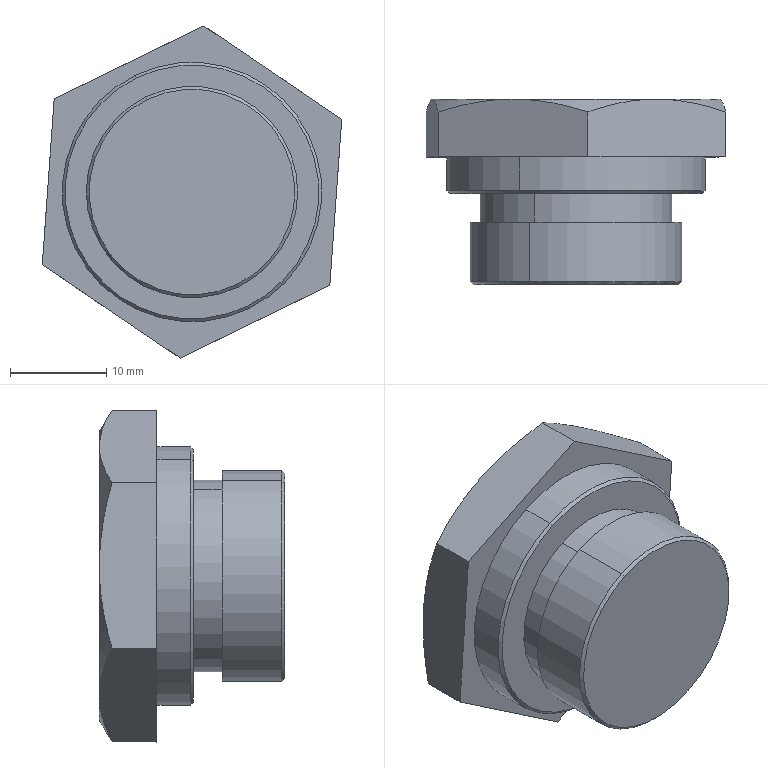Part | SolidWorks | features BaseBody 1 | 1 solid | 27 faces | box 31.164 x 19.3 x 34.552 mm | volume 10229 mm3 | plane 11 | cone 10 | cylinder 6 | commonest cylinder face diameters 20 x2 22 x2 27 x2
STEP:
#1=CARTESIAN_POINT('',(-39.66,84.896,-168.446));
#2=VERTEX_POINT('',#1);
#3=CARTESIAN_POINT('',(-49.266,84.896,-148.654));
#4=VERTEX_POINT('',#3);
#5=CARTESIAN_POINT('',(-44.463,84.896,-158.55));
#6=DIRECTION('',(0.,1.,0.));
#7=DIRECTION('',(0.4367,0.,-0.8996));
#8=AXIS2_PLACEMENT_3D('',#5,#6,#7);
#9=CIRCLE('',#8,11.);
#10=EDGE_CURVE('',#2,#4,#9,.T.);
#11=ORIENTED_EDGE('',*,*,#10,.T.);
#12=CARTESIAN_POINT('',(-49.266,91.096,-148.654));
#13=VERTEX_POINT('',#12);
#14=CARTESIAN_POINT('',(-49.266,153.67,-148.654));
#15=DIRECTION('',(0.,1.,0.));
#16=VECTOR('',#15,1000.);
#17=LINE('',#14,#16);
#18=EDGE_CURVE('',#4,#13,#17,.T.);
#19=ORIENTED_EDGE('',*,*,#18,.T.);
#20=CARTESIAN_POINT('',(-39.66,91.096,-168.446));
#21=VERTEX_POINT('',#20);
#22=CARTESIAN_POINT('',(-44.463,91.096,-158.55));
#23=DIRECTION('',(0.,1.,0.));
#24=DIRECTION('',(0.4367,0.,-0.8996));
#25=AXIS2_PLACEMENT_3D('',#22,#23,#24);
#26=CIRCLE('',#25,11.);
#27=EDGE_CURVE('',#21,#13,#26,.T.);
#28=ORIENTED_EDGE('',*,*,#27,.F.);
#29=CARTESIAN_POINT('',(-39.66,153.67,-168.446));
#30=DIRECTION('',(0.,1.,0.));
#31=VECTOR('',#30,1000.);
#32=LINE('',#29,#31);
#33=EDGE_CURVE('',#2,#21,#32,.T.);
#34=ORIENTED_EDGE('',*,*,#33,.F.);
#35=EDGE_LOOP('',(#11,#19,#28,#34));
#36=FACE_OUTER_BOUND('',#35,.T.);
#37=CARTESIAN_POINT('',(-44.463,153.67,-158.55));
#38=DIRECTION('',(0.,1.,0.));
#39=DIRECTION('',(0.4367,0.,-0.8996));
#40=AXIS2_PLACEMENT_3D('',#37,#38,#39);
#41=CYLINDRICAL_SURFACE('',#40,11.);
#42=ADVANCED_FACE('',(#36),#41,.T.);
#43=CARTESIAN_POINT('',(-40.096,91.096,-167.546));
#44=VERTEX_POINT('',#43);
#45=CARTESIAN_POINT('',(-48.829,91.096,-149.554));
#46=VERTEX_POINT('',#45);
#47=CARTESIAN_POINT('',(-44.463,91.096,-158.55));
#48=DIRECTION('',(0.,1.,0.));
#49=DIRECTION('',(0.4367,0.,-0.8996));
#50=AXIS2_PLACEMENT_3D('',#47,#48,#49);
#51=CIRCLE('',#50,10.);
#52=EDGE_CURVE('',#44,#46,#51,.T.);
#53=ORIENTED_EDGE('',*,*,#52,.T.);
#54=CARTESIAN_POINT('',(-48.829,94.096,-149.554));
#55=VERTEX_POINT('',#54);
#56=CARTESIAN_POINT('',(-48.829,153.67,-149.554));
#57=DIRECTION('',(0.,1.,0.));
#58=VECTOR('',#57,1000.);
#59=LINE('',#56,#58);
#60=EDGE_CURVE('',#46,#55,#59,.T.);
#61=ORIENTED_EDGE('',*,*,#60,.T.);
#62=CARTESIAN_POINT('',(-40.096,94.096,-167.546));
#63=VERTEX_POINT('',#62);
#64=CARTESIAN_POINT('',(-44.463,94.096,-158.55));
#65=DIRECTION('',(0.,1.,0.));
#66=DIRECTION('',(0.4367,0.,-0.8996));
#67=AXIS2_PLACEMENT_3D('',#64,#65,#66);
#68=CIRCLE('',#67,10.);
#69=EDGE_CURVE('',#63,#55,#68,.T.);
#70=ORIENTED_EDGE('',*,*,#69,.F.);
#71=CARTESIAN_POINT('',(-40.096,153.67,-167.546));
#72=DIRECTION('',(0.,1.,0.));
#73=VECTOR('',#72,1000.);
#74=LINE('',#71,#73);
#75=EDGE_CURVE('',#44,#63,#74,.T.);
#76=ORIENTED_EDGE('',*,*,#75,.F.);
#77=EDGE_LOOP('',(#53,#61,#70,#76));
#78=FACE_OUTER_BOUND('',#77,.T.);
#79=CARTESIAN_POINT('',(-44.463,153.67,-158.55));
#80=DIRECTION('',(0.,1.,0.));
#81=DIRECTION('',(0.4367,0.,-0.8996));
#82=AXIS2_PLACEMENT_3D('',#79,#80,#81);
#83=CYLINDRICAL_SURFACE('',#82,10.);
#84=ADVANCED_FACE('',(#78),#83,.T.);
#85=CARTESIAN_POINT('',(-38.699,94.096,-170.425));
#86=VERTEX_POINT('',#85);
#87=CARTESIAN_POINT('',(-50.227,94.096,-146.675));
#88=VERTEX_POINT('',#87);
#89=CARTESIAN_POINT('',(-44.463,94.096,-158.55));
#90=DIRECTION('',(0.,1.,0.));
#91=DIRECTION('',(0.4367,0.,-0.8996));
#92=AXIS2_PLACEMENT_3D('',#89,#90,#91);
#93=CIRCLE('',#92,13.2);
#94=EDGE_CURVE('',#86,#88,#93,.T.);
#95=ORIENTED_EDGE('',*,*,#94,.T.);
#96=CARTESIAN_POINT('',(-50.358,94.396,-146.405));
#97=VERTEX_POINT('',#96);
#98=CARTESIAN_POINT('',(-50.227,94.096,-146.675));
#99=DIRECTION('',(-0.3088,0.7071,0.6361));
#100=VECTOR('',#99,1000.);
#101=LINE('',#98,#100);
#102=EDGE_CURVE('',#88,#97,#101,.T.);
#103=ORIENTED_EDGE('',*,*,#102,.T.);
#104=CARTESIAN_POINT('',(-38.568,94.396,-170.695));
#105=VERTEX_POINT('',#104);
#106=CARTESIAN_POINT('',(-44.463,94.396,-158.55));
#107=DIRECTION('',(0.,1.,0.));
#108=DIRECTION('',(0.4367,0.,-0.8996));
#109=AXIS2_PLACEMENT_3D('',#106,#107,#108);
#110=CIRCLE('',#109,13.5);
#111=EDGE_CURVE('',#105,#97,#110,.T.);
#112=ORIENTED_EDGE('',*,*,#111,.F.);
#113=CARTESIAN_POINT('',(-38.699,94.096,-170.425));
#114=DIRECTION('',(0.3088,0.7071,-0.6361));
#115=VECTOR('',#114,1000.);
#116=LINE('',#113,#115);
#117=EDGE_CURVE('',#86,#105,#116,.T.);
#118=ORIENTED_EDGE('',*,*,#117,.F.);
#119=EDGE_LOOP('',(#95,#103,#112,#118));
#120=FACE_OUTER_BOUND('',#119,.T.);
#121=CARTESIAN_POINT('',(-44.463,94.096,-158.55));
#122=DIRECTION('',(0.,1.,0.));
#123=DIRECTION('',(0.4367,0.,-0.8996));
#124=AXIS2_PLACEMENT_3D('',#121,#122,#123);
#125=CONICAL_SURFACE('',#124,13.2,0.7854);
#126=ADVANCED_FACE('',(#120),#125,.T.);
#127=ORIENTED_EDGE('',*,*,#111,.T.);
#128=CARTESIAN_POINT('',(-50.358,97.896,-146.405));
#129=VERTEX_POINT('',#128);
#130=CARTESIAN_POINT('',(-50.358,153.67,-146.405));
#131=DIRECTION('',(0.,1.,0.));
#132=VECTOR('',#131,1000.);
#133=LINE('',#130,#132);
#134=EDGE_CURVE('',#97,#129,#133,.T.);
#135=ORIENTED_EDGE('',*,*,#134,.T.);
#136=CARTESIAN_POINT('',(-38.568,97.896,-170.695));
#137=VERTEX_POINT('',#136);
#138=CARTESIAN_POINT('',(-44.463,97.896,-158.55));
#139=DIRECTION('',(0.,1.,0.));
#140=DIRECTION('',(0.4367,0.,-0.8996));
#141=AXIS2_PLACEMENT_3D('',#138,#139,#140);
#142=CIRCLE('',#141,13.5);
#143=EDGE_CURVE('',#137,#129,#142,.T.);
#144=ORIENTED_EDGE('',*,*,#143,.F.);
#145=CARTESIAN_POINT('',(-38.568,153.67,-170.695));
#146=DIRECTION('',(0.,1.,0.));
#147=VECTOR('',#146,1000.);
#148=LINE('',#145,#147);
#149=EDGE_CURVE('',#105,#137,#148,.T.);
#150=ORIENTED_EDGE('',*,*,#149,.F.);
#151=EDGE_LOOP('',(#127,#135,#144,#150));
#152=FACE_OUTER_BOUND('',#151,.T.);
#153=CARTESIAN_POINT('',(-44.463,153.67,-158.55));
#154=DIRECTION('',(0.,1.,0.));
#155=DIRECTION('',(0.4367,0.,-0.8996));
#156=AXIS2_PLACEMENT_3D('',#153,#154,#155);
#157=CYLINDRICAL_SURFACE('',#156,13.5);
#158=ADVANCED_FACE('',(#152),#157,.T.);
#159=CARTESIAN_POINT('',(-49.135,84.596,-148.924));
#160=VERTEX_POINT('',#159);
#161=CARTESIAN_POINT('',(-39.791,84.596,-168.176));
#162=VERTEX_POINT('',#161);
#163=CARTESIAN_POINT('',(-44.463,84.596,-158.55));
#164=DIRECTION('',(0.,-1.,0.));
#165=DIRECTION('',(0.4367,0.,-0.8996));
#166=AXIS2_PLACEMENT_3D('',#163,#164,#165);
#167=CIRCLE('',#166,10.7);
#168=EDGE_CURVE('',#160,#162,#167,.T.);
#169=ORIENTED_EDGE('',*,*,#168,.F.);
#170=CARTESIAN_POINT('',(-49.266,84.896,-148.654));
#171=DIRECTION('',(-0.3088,0.7071,0.6361));
#172=VECTOR('',#171,1000.);
#173=LINE('',#170,#172);
#174=EDGE_CURVE('',#160,#4,#173,.T.);
#175=ORIENTED_EDGE('',*,*,#174,.T.);
#176=ORIENTED_EDGE('',*,*,#10,.F.);
#177=CARTESIAN_POINT('',(-39.66,84.896,-168.446));
#178=DIRECTION('',(0.3088,0.7071,-0.6361));
#179=VECTOR('',#178,1000.);
#180=LINE('',#177,#179);
#181=EDGE_CURVE('',#162,#2,#180,.T.);
#182=ORIENTED_EDGE('',*,*,#181,.F.);
#183=EDGE_LOOP('',(#169,#175,#176,#182));
#184=FACE_OUTER_BOUND('',#183,.T.);
#185=CARTESIAN_POINT('',(-44.463,84.896,-158.55));
#186=DIRECTION('',(0.,1.,0.));
#187=DIRECTION('',(0.4367,0.,-0.8996));
#188=AXIS2_PLACEMENT_3D('',#185,#186,#187);
#189=CONICAL_SURFACE('',#188,11.,0.7854);
#190=ADVANCED_FACE('',(#184),#189,.T.);
#191=ORIENTED_EDGE('',*,*,#174,.F.);
#192=CARTESIAN_POINT('',(-44.463,84.596,-158.55));
#193=DIRECTION('',(0.,-1.,0.));
#194=DIRECTION('',(0.4367,0.,-0.8996));
#195=AXIS2_PLACEMENT_3D('',#192,#193,#194);
#196=CIRCLE('',#195,10.7);
#197=EDGE_CURVE('',#162,#160,#196,.T.);
#198=ORIENTED_EDGE('',*,*,#197,.F.);
#199=ORIENTED_EDGE('',*,*,#181,.T.);
#200=CARTESIAN_POINT('',(-44.463,84.896,-158.55));
#201=DIRECTION('',(0.,1.,0.));
#202=DIRECTION('',(0.4367,0.,-0.8996));
#203=AXIS2_PLACEMENT_3D('',#200,#201,#202);
#204=CIRCLE('',#203,11.);
#205=EDGE_CURVE('',#4,#2,#204,.T.);
#206=ORIENTED_EDGE('',*,*,#205,.F.);
#207=EDGE_LOOP('',(#191,#198,#199,#206));
#208=FACE_OUTER_BOUND('',#207,.T.);
#209=CARTESIAN_POINT('',(-44.463,84.896,-158.55));
#210=DIRECTION('',(0.,1.,0.));
#211=DIRECTION('',(0.4367,0.,-0.8996));
#212=AXIS2_PLACEMENT_3D('',#209,#210,#211);
#213=CONICAL_SURFACE('',#212,11.,0.7854);
#214=ADVANCED_FACE('',(#208),#213,.T.);
#215=CARTESIAN_POINT('',(-51.013,103.896,-145.056));
#216=VERTEX_POINT('',#215);
#217=CARTESIAN_POINT('',(-59.424,103.896,-157.475));
#218=VERTEX_POINT('',#217);
#219=CARTESIAN_POINT('',(-44.463,103.896,-158.55));
#220=DIRECTION('',(0.,-1.,0.));
#221=DIRECTION('',(-0.4367,0.,0.8996));
#222=AXIS2_PLACEMENT_3D('',#219,#220,#221);
#223=CIRCLE('',#222,15.);
#224=EDGE_CURVE('',#216,#218,#223,.T.);
#225=ORIENTED_EDGE('',*,*,#224,.F.);
#226=CARTESIAN_POINT('',(-36.051,103.896,-146.13));
#227=VERTEX_POINT('',#226);
#228=CARTESIAN_POINT('',(-44.463,103.896,-158.55));
#229=DIRECTION('',(0.,-1.,0.));
#230=DIRECTION('',(-0.4367,0.,0.8996));
#231=AXIS2_PLACEMENT_3D('',#228,#229,#230);
#232=CIRCLE('',#231,15.);
#233=EDGE_CURVE('',#227,#216,#232,.T.);
#234=ORIENTED_EDGE('',*,*,#233,.F.);
#235=CARTESIAN_POINT('',(-29.501,103.896,-159.625));
#236=VERTEX_POINT('',#235);
#237=CARTESIAN_POINT('',(-44.463,103.896,-158.55));
#238=DIRECTION('',(0.,-1.,0.));
#239=DIRECTION('',(-0.4367,0.,0.8996));
#240=AXIS2_PLACEMENT_3D('',#237,#238,#239);
#241=CIRCLE('',#240,15.);
#242=EDGE_CURVE('',#236,#227,#241,.T.);
#243=ORIENTED_EDGE('',*,*,#242,.F.);
#244=CARTESIAN_POINT('',(-37.913,103.896,-172.044));
#245=VERTEX_POINT('',#244);
#246=CARTESIAN_POINT('',(-44.463,103.896,-158.55));
#247=DIRECTION('',(0.,-1.,0.));
#248=DIRECTION('',(-0.4367,0.,0.8996));
#249=AXIS2_PLACEMENT_3D('',#246,#247,#248);
#250=CIRCLE('',#249,15.);
#251=EDGE_CURVE('',#245,#236,#250,.T.);
#252=ORIENTED_EDGE('',*,*,#251,.F.);
#253=CARTESIAN_POINT('',(-52.874,103.896,-170.97));
#254=VERTEX_POINT('',#253);
#255=CARTESIAN_POINT('',(-44.463,103.896,-158.55));
#256=DIRECTION('',(0.,1.,0.));
#257=DIRECTION('',(0.4367,0.,-0.8996));
#258=AXIS2_PLACEMENT_3D('',#255,#256,#257);
#259=CIRCLE('',#258,15.);
#260=EDGE_CURVE('',#245,#254,#259,.T.);
#261=ORIENTED_EDGE('',*,*,#260,.T.);
#262=CARTESIAN_POINT('',(-44.463,103.896,-158.55));
#263=DIRECTION('',(0.,-1.,0.));
#264=DIRECTION('',(-0.4367,0.,0.8996));
#265=AXIS2_PLACEMENT_3D('',#262,#263,#264);
#266=CIRCLE('',#265,15.);
#267=EDGE_CURVE('',#218,#254,#266,.T.);
#268=ORIENTED_EDGE('',*,*,#267,.F.);
#269=EDGE_LOOP('',(#225,#234,#243,#252,#261,#268));
#270=FACE_OUTER_BOUND('',#269,.T.);
#271=CARTESIAN_POINT('',(-44.463,103.896,-158.55));
#272=DIRECTION('',(0.,-1.,0.));
#273=DIRECTION('',(-1.,0.,0.));
#274=AXIS2_PLACEMENT_3D('',#271,#272,#273);
#275=PLANE('',#274);
#276=ADVANCED_FACE('',(#270),#275,.F.);
#277=ORIENTED_EDGE('',*,*,#224,.T.);
#278=CARTESIAN_POINT('',(-58.804,102.556,-148.837));
#279=VERTEX_POINT('',#278);
#280=CARTESIAN_POINT('',(-58.804,102.556,-148.837));
#281=CARTESIAN_POINT('',(-58.905,102.965,-150.248));
#282=CARTESIAN_POINT('',(-59.007,103.302,-151.67));
#283=CARTESIAN_POINT('',(-59.214,103.768,-154.547));
#284=CARTESIAN_POINT('',(-59.318,103.896,-156.001));
#285=CARTESIAN_POINT('',(-59.424,103.896,-157.475));
#286=B_SPLINE_CURVE_WITH_KNOTS('',3,(#280,#281,#282,#283,#284,#285),.UNSPECIFIED.,.F.,.F.,(4,2,4),(0.,0.004382,0.008763),.UNSPECIFIED.);
#287=EDGE_CURVE('',#279,#218,#286,.T.);
#288=ORIENTED_EDGE('',*,*,#287,.F.);
#289=CARTESIAN_POINT('',(-51.013,103.896,-145.056));
#290=CARTESIAN_POINT('',(-52.342,103.896,-145.701));
#291=CARTESIAN_POINT('',(-53.654,103.768,-146.338));
#292=CARTESIAN_POINT('',(-56.248,103.302,-147.597));
#293=CARTESIAN_POINT('',(-57.531,102.965,-148.219));
#294=CARTESIAN_POINT('',(-58.804,102.556,-148.837));
#295=B_SPLINE_CURVE_WITH_KNOTS('',3,(#289,#290,#291,#292,#293,#294),.UNSPECIFIED.,.F.,.F.,(4,2,4),(0.,0.004382,0.008763),.UNSPECIFIED.);
#296=EDGE_CURVE('',#216,#279,#295,.T.);
#297=ORIENTED_EDGE('',*,*,#296,.F.);
#298=EDGE_LOOP('',(#277,#288,#297));
#299=FACE_OUTER_BOUND('',#298,.T.);
#300=CARTESIAN_POINT('',(-44.463,103.896,-158.55));
#301=DIRECTION('',(0.,-1.,0.));
#302=DIRECTION('',(-0.4367,0.,0.8996));
#303=AXIS2_PLACEMENT_3D('',#300,#301,#302);
#304=CONICAL_SURFACE('',#303,15.,1.047);
#305=ADVANCED_FACE('',(#299),#304,.T.);
#306=CARTESIAN_POINT('',(-60.045,102.556,-166.113));
#307=VERTEX_POINT('',#306);
#308=CARTESIAN_POINT('',(-59.424,103.896,-157.475));
#309=CARTESIAN_POINT('',(-59.53,103.896,-158.949));
#310=CARTESIAN_POINT('',(-59.635,103.768,-160.404));
#311=CARTESIAN_POINT('',(-59.841,103.302,-163.28));
#312=CARTESIAN_POINT('',(-59.944,102.965,-164.702));
#313=CARTESIAN_POINT('',(-60.045,102.556,-166.113));
#314=B_SPLINE_CURVE_WITH_KNOTS('',3,(#308,#309,#310,#311,#312,#313),.UNSPECIFIED.,.F.,.F.,(4,2,4),(0.,0.004382,0.008763),.UNSPECIFIED.);
#315=EDGE_CURVE('',#218,#307,#314,.T.);
#316=ORIENTED_EDGE('',*,*,#315,.F.);
#317=ORIENTED_EDGE('',*,*,#267,.T.);
#318=CARTESIAN_POINT('',(-60.045,102.556,-166.113));
#319=CARTESIAN_POINT('',(-58.874,102.965,-166.906));
#320=CARTESIAN_POINT('',(-57.693,103.302,-167.706));
#321=CARTESIAN_POINT('',(-55.305,103.768,-169.323));
#322=CARTESIAN_POINT('',(-54.098,103.896,-170.141));
#323=CARTESIAN_POINT('',(-52.874,103.896,-170.97));
#324=B_SPLINE_CURVE_WITH_KNOTS('',3,(#318,#319,#320,#321,#322,#323),.UNSPECIFIED.,.F.,.F.,(4,2,4),(0.,0.004382,0.008763),.UNSPECIFIED.);
#325=EDGE_CURVE('',#307,#254,#324,.T.);
#326=ORIENTED_EDGE('',*,*,#325,.F.);
#327=EDGE_LOOP('',(#316,#317,#326));
#328=FACE_OUTER_BOUND('',#327,.T.);
#329=CARTESIAN_POINT('',(-44.463,103.896,-158.55));
#330=DIRECTION('',(0.,-1.,0.));
#331=DIRECTION('',(-0.4367,0.,0.8996));
#332=AXIS2_PLACEMENT_3D('',#329,#330,#331);
#333=CONICAL_SURFACE('',#332,15.,1.047);
#334=ADVANCED_FACE('',(#328),#333,.T.);
#335=ORIENTED_EDGE('',*,*,#260,.F.);
#336=CARTESIAN_POINT('',(-45.704,102.556,-175.826));
#337=VERTEX_POINT('',#336);
#338=CARTESIAN_POINT('',(-45.704,102.556,-175.826));
#339=CARTESIAN_POINT('',(-44.431,102.965,-175.208));
#340=CARTESIAN_POINT('',(-43.149,103.302,-174.586));
#341=CARTESIAN_POINT('',(-40.554,103.768,-173.326));
#342=CARTESIAN_POINT('',(-39.243,103.896,-172.69));
#343=CARTESIAN_POINT('',(-37.913,103.896,-172.044));
#344=B_SPLINE_CURVE_WITH_KNOTS('',3,(#338,#339,#340,#341,#342,#343),.UNSPECIFIED.,.F.,.F.,(4,2,4),(0.,0.004382,0.008763),.UNSPECIFIED.);
#345=EDGE_CURVE('',#337,#245,#344,.T.);
#346=ORIENTED_EDGE('',*,*,#345,.F.);
#347=CARTESIAN_POINT('',(-52.874,103.896,-170.97));
#348=CARTESIAN_POINT('',(-51.651,103.896,-171.798));
#349=CARTESIAN_POINT('',(-50.444,103.768,-172.616));
#350=CARTESIAN_POINT('',(-48.056,103.302,-174.233));
#351=CARTESIAN_POINT('',(-46.875,102.965,-175.033));
#352=CARTESIAN_POINT('',(-45.704,102.556,-175.826));
#353=B_SPLINE_CURVE_WITH_KNOTS('',3,(#347,#348,#349,#350,#351,#352),.UNSPECIFIED.,.F.,.F.,(4,2,4),(0.,0.004382,0.008763),.UNSPECIFIED.);
#354=EDGE_CURVE('',#254,#337,#353,.T.);
#355=ORIENTED_EDGE('',*,*,#354,.F.);
#356=EDGE_LOOP('',(#335,#346,#355));
#357=FACE_OUTER_BOUND('',#356,.T.);
#358=CARTESIAN_POINT('',(-44.463,103.896,-158.55));
#359=DIRECTION('',(0.,-1.,0.));
#360=DIRECTION('',(-0.4367,0.,0.8996));
#361=AXIS2_PLACEMENT_3D('',#358,#359,#360);
#362=CONICAL_SURFACE('',#361,15.,1.047);
#363=ADVANCED_FACE('',(#357),#362,.T.);
#364=ORIENTED_EDGE('',*,*,#251,.T.);
#365=CARTESIAN_POINT('',(-30.122,102.556,-168.263));
#366=VERTEX_POINT('',#365);
#367=CARTESIAN_POINT('',(-30.122,102.556,-168.263));
#368=CARTESIAN_POINT('',(-30.021,102.965,-166.852));
#369=CARTESIAN_POINT('',(-29.918,103.302,-165.43));
#370=CARTESIAN_POINT('',(-29.712,103.768,-162.553));
#371=CARTESIAN_POINT('',(-29.607,103.896,-161.099));
#372=CARTESIAN_POINT('',(-29.501,103.896,-159.625));
#373=B_SPLINE_CURVE_WITH_KNOTS('',3,(#367,#368,#369,#370,#371,#372),.UNSPECIFIED.,.F.,.F.,(4,2,4),(0.,0.004382,0.008763),.UNSPECIFIED.);
#374=EDGE_CURVE('',#366,#236,#373,.T.);
#375=ORIENTED_EDGE('',*,*,#374,.F.);
#376=CARTESIAN_POINT('',(-37.913,103.896,-172.044));
#377=CARTESIAN_POINT('',(-36.583,103.896,-171.399));
#378=CARTESIAN_POINT('',(-35.272,103.768,-170.762));
#379=CARTESIAN_POINT('',(-32.677,103.302,-169.503));
#380=CARTESIAN_POINT('',(-31.395,102.965,-168.881));
#381=CARTESIAN_POINT('',(-30.122,102.556,-168.263));
#382=B_SPLINE_CURVE_WITH_KNOTS('',3,(#376,#377,#378,#379,#380,#381),.UNSPECIFIED.,.F.,.F.,(4,2,4),(0.,0.004382,0.008763),.UNSPECIFIED.);
#383=EDGE_CURVE('',#245,#366,#382,.T.);
#384=ORIENTED_EDGE('',*,*,#383,.F.);
#385=EDGE_LOOP('',(#364,#375,#384));
#386=FACE_OUTER_BOUND('',#385,.T.);
#387=CARTESIAN_POINT('',(-44.463,103.896,-158.55));
#388=DIRECTION('',(0.,-1.,0.));
#389=DIRECTION('',(-0.4367,0.,0.8996));
#390=AXIS2_PLACEMENT_3D('',#387,#388,#389);
#391=CONICAL_SURFACE('',#390,15.,1.047);
#392=ADVANCED_FACE('',(#386),#391,.T.);
#393=ORIENTED_EDGE('',*,*,#242,.T.);
#394=CARTESIAN_POINT('',(-28.881,102.556,-150.987));
#395=VERTEX_POINT('',#394);
#396=CARTESIAN_POINT('',(-28.881,102.556,-150.987));
#397=CARTESIAN_POINT('',(-30.052,102.965,-150.194));
#398=CARTESIAN_POINT('',(-31.233,103.302,-149.394));
#399=CARTESIAN_POINT('',(-33.62,103.768,-147.777));
#400=CARTESIAN_POINT('',(-34.828,103.896,-146.959));
#401=CARTESIAN_POINT('',(-36.051,103.896,-146.13));
#402=B_SPLINE_CURVE_WITH_KNOTS('',3,(#396,#397,#398,#399,#400,#401),.UNSPECIFIED.,.F.,.F.,(4,2,4),(0.,0.004382,0.008763),.UNSPECIFIED.);
#403=EDGE_CURVE('',#395,#227,#402,.T.);
#404=ORIENTED_EDGE('',*,*,#403,.F.);
#405=CARTESIAN_POINT('',(-29.501,103.896,-159.625));
#406=CARTESIAN_POINT('',(-29.396,103.896,-158.151));
#407=CARTESIAN_POINT('',(-29.291,103.768,-156.696));
#408=CARTESIAN_POINT('',(-29.084,103.302,-153.82));
#409=CARTESIAN_POINT('',(-28.982,102.965,-152.398));
#410=CARTESIAN_POINT('',(-28.881,102.556,-150.987));
#411=B_SPLINE_CURVE_WITH_KNOTS('',3,(#405,#406,#407,#408,#409,#410),.UNSPECIFIED.,.F.,.F.,(4,2,4),(0.,0.004382,0.008763),.UNSPECIFIED.);
#412=EDGE_CURVE('',#236,#395,#411,.T.);
#413=ORIENTED_EDGE('',*,*,#412,.F.);
#414=EDGE_LOOP('',(#393,#404,#413));
#415=FACE_OUTER_BOUND('',#414,.T.);
#416=CARTESIAN_POINT('',(-44.463,103.896,-158.55));
#417=DIRECTION('',(0.,-1.,0.));
#418=DIRECTION('',(-0.4367,0.,0.8996));
#419=AXIS2_PLACEMENT_3D('',#416,#417,#418);
#420=CONICAL_SURFACE('',#419,15.,1.047);
#421=ADVANCED_FACE('',(#415),#420,.T.);
#422=ORIENTED_EDGE('',*,*,#233,.T.);
#423=CARTESIAN_POINT('',(-43.222,102.556,-141.274));
#424=VERTEX_POINT('',#423);
#425=CARTESIAN_POINT('',(-43.222,102.556,-141.274));
#426=CARTESIAN_POINT('',(-44.494,102.965,-141.892));
#427=CARTESIAN_POINT('',(-45.777,103.302,-142.514));
#428=CARTESIAN_POINT('',(-48.371,103.768,-143.774));
#429=CARTESIAN_POINT('',(-49.683,103.896,-144.41));
#430=CARTESIAN_POINT('',(-51.013,103.896,-145.056));
#431=B_SPLINE_CURVE_WITH_KNOTS('',3,(#425,#426,#427,#428,#429,#430),.UNSPECIFIED.,.F.,.F.,(4,2,4),(0.,0.004382,0.008763),.UNSPECIFIED.);
#432=EDGE_CURVE('',#424,#216,#431,.T.);
#433=ORIENTED_EDGE('',*,*,#432,.F.);
#434=CARTESIAN_POINT('',(-36.051,103.896,-146.13));
#435=CARTESIAN_POINT('',(-37.275,103.896,-145.302));
#436=CARTESIAN_POINT('',(-38.482,103.768,-144.484));
#437=CARTESIAN_POINT('',(-40.87,103.302,-142.867));
#438=CARTESIAN_POINT('',(-42.05,102.965,-142.067));
#439=CARTESIAN_POINT('',(-43.222,102.556,-141.274));
#440=B_SPLINE_CURVE_WITH_KNOTS('',3,(#434,#435,#436,#437,#438,#439),.UNSPECIFIED.,.F.,.F.,(4,2,4),(0.,0.004382,0.008763),.UNSPECIFIED.);
#441=EDGE_CURVE('',#227,#424,#440,.T.);
#442=ORIENTED_EDGE('',*,*,#441,.F.);
#443=EDGE_LOOP('',(#422,#433,#442));
#444=FACE_OUTER_BOUND('',#443,.T.);
#445=CARTESIAN_POINT('',(-44.463,103.896,-158.55));
#446=DIRECTION('',(0.,-1.,0.));
#447=DIRECTION('',(-0.4367,0.,0.8996));
#448=AXIS2_PLACEMENT_3D('',#445,#446,#447);
#449=CONICAL_SURFACE('',#448,15.,1.047);
#450=ADVANCED_FACE('',(#444),#449,.T.);
#451=ORIENTED_EDGE('',*,*,#143,.T.);
#452=CARTESIAN_POINT('',(-44.463,97.896,-158.55));
#453=DIRECTION('',(0.,1.,0.));
#454=DIRECTION('',(0.4367,0.,-0.8996));
#455=AXIS2_PLACEMENT_3D('',#452,#453,#454);
#456=CIRCLE('',#455,13.5);
#457=EDGE_CURVE('',#129,#137,#456,.T.);
#458=ORIENTED_EDGE('',*,*,#457,.T.);
#459=EDGE_LOOP('',(#451,#458));
#460=FACE_BOUND('',#459,.T.);
#461=CARTESIAN_POINT('',(-58.804,97.896,-148.837));
#462=VERTEX_POINT('',#461);
#463=CARTESIAN_POINT('',(-60.045,97.896,-166.113));
#464=VERTEX_POINT('',#463);
#465=CARTESIAN_POINT('',(-60.045,97.896,-166.113));
#466=DIRECTION('',(-0.07166,0.,-0.9974));
#467=VECTOR('',#466,1000.);
#468=LINE('',#465,#467);
#469=EDGE_CURVE('',#462,#464,#468,.T.);
#470=ORIENTED_EDGE('',*,*,#469,.T.);
#471=CARTESIAN_POINT('',(-45.704,97.896,-175.826));
#472=VERTEX_POINT('',#471);
#473=CARTESIAN_POINT('',(-45.704,97.896,-175.826));
#474=DIRECTION('',(0.828,0.,-0.5608));
#475=VECTOR('',#474,1000.);
#476=LINE('',#473,#475);
#477=EDGE_CURVE('',#464,#472,#476,.T.);
#478=ORIENTED_EDGE('',*,*,#477,.T.);
#479=CARTESIAN_POINT('',(-30.122,97.896,-168.263));
#480=VERTEX_POINT('',#479);
#481=CARTESIAN_POINT('',(-30.122,97.896,-168.263));
#482=DIRECTION('',(0.8996,0.,0.4367));
#483=VECTOR('',#482,1000.);
#484=LINE('',#481,#483);
#485=EDGE_CURVE('',#472,#480,#484,.T.);
#486=ORIENTED_EDGE('',*,*,#485,.T.);
#487=CARTESIAN_POINT('',(-28.881,97.896,-150.987));
#488=VERTEX_POINT('',#487);
#489=CARTESIAN_POINT('',(-28.881,97.896,-150.987));
#490=DIRECTION('',(0.07166,0.,0.9974));
#491=VECTOR('',#490,1000.);
#492=LINE('',#489,#491);
#493=EDGE_CURVE('',#480,#488,#492,.T.);
#494=ORIENTED_EDGE('',*,*,#493,.T.);
#495=CARTESIAN_POINT('',(-43.222,97.896,-141.274));
#496=VERTEX_POINT('',#495);
#497=CARTESIAN_POINT('',(-43.222,97.896,-141.274));
#498=DIRECTION('',(-0.828,0.,0.5608));
#499=VECTOR('',#498,1000.);
#500=LINE('',#497,#499);
#501=EDGE_CURVE('',#488,#496,#500,.T.);
#502=ORIENTED_EDGE('',*,*,#501,.T.);
#503=CARTESIAN_POINT('',(-58.804,97.896,-148.837));
#504=DIRECTION('',(-0.8996,0.,-0.4367));
#505=VECTOR('',#504,1000.);
#506=LINE('',#503,#505);
#507=EDGE_CURVE('',#496,#462,#506,.T.);
#508=ORIENTED_EDGE('',*,*,#507,.T.);
#509=EDGE_LOOP('',(#470,#478,#486,#494,#502,#508));
#510=FACE_OUTER_BOUND('',#509,.T.);
#511=CARTESIAN_POINT('',(-57.957,97.896,-165.1));
#512=DIRECTION('',(0.,1.,0.));
#513=DIRECTION('',(1.,0.,0.));
#514=AXIS2_PLACEMENT_3D('',#511,#512,#513);
#515=PLANE('',#514);
#516=ADVANCED_FACE('',(#460,#510),#515,.F.);
#517=ORIENTED_EDGE('',*,*,#134,.F.);
#518=CARTESIAN_POINT('',(-44.463,94.396,-158.55));
#519=DIRECTION('',(0.,1.,0.));
#520=DIRECTION('',(0.4367,0.,-0.8996));
#521=AXIS2_PLACEMENT_3D('',#518,#519,#520);
#522=CIRCLE('',#521,13.5);
#523=EDGE_CURVE('',#97,#105,#522,.T.);
#524=ORIENTED_EDGE('',*,*,#523,.T.);
#525=ORIENTED_EDGE('',*,*,#149,.T.);
#526=ORIENTED_EDGE('',*,*,#457,.F.);
#527=EDGE_LOOP('',(#517,#524,#525,#526));
#528=FACE_OUTER_BOUND('',#527,.T.);
#529=CARTESIAN_POINT('',(-44.463,153.67,-158.55));
#530=DIRECTION('',(0.,1.,0.));
#531=DIRECTION('',(0.4367,0.,-0.8996));
#532=AXIS2_PLACEMENT_3D('',#529,#530,#531);
#533=CYLINDRICAL_SURFACE('',#532,13.5);
#534=ADVANCED_FACE('',(#528),#533,.T.);
#535=ORIENTED_EDGE('',*,*,#102,.F.);
#536=CARTESIAN_POINT('',(-44.463,94.096,-158.55));
#537=DIRECTION('',(0.,1.,0.));
#538=DIRECTION('',(0.4367,0.,-0.8996));
#539=AXIS2_PLACEMENT_3D('',#536,#537,#538);
#540=CIRCLE('',#539,13.2);
#541=EDGE_CURVE('',#88,#86,#540,.T.);
#542=ORIENTED_EDGE('',*,*,#541,.T.);
#543=ORIENTED_EDGE('',*,*,#117,.T.);
#544=ORIENTED_EDGE('',*,*,#523,.F.);
#545=EDGE_LOOP('',(#535,#542,#543,#544));
#546=FACE_OUTER_BOUND('',#545,.T.);
#547=CARTESIAN_POINT('',(-44.463,94.096,-158.55));
#548=DIRECTION('',(0.,1.,0.));
#549=DIRECTION('',(0.4367,0.,-0.8996));
#550=AXIS2_PLACEMENT_3D('',#547,#548,#549);
#551=CONICAL_SURFACE('',#550,13.2,0.7854);
#552=ADVANCED_FACE('',(#546),#551,.T.);
#553=ORIENTED_EDGE('',*,*,#69,.T.);
#554=CARTESIAN_POINT('',(-44.463,94.096,-158.55));
#555=DIRECTION('',(0.,1.,0.));
#556=DIRECTION('',(0.4367,0.,-0.8996));
#557=AXIS2_PLACEMENT_3D('',#554,#555,#556);
#558=CIRCLE('',#557,10.);
#559=EDGE_CURVE('',#55,#63,#558,.T.);
#560=ORIENTED_EDGE('',*,*,#559,.T.);
#561=EDGE_LOOP('',(#553,#560));
#562=FACE_BOUND('',#561,.T.);
#563=ORIENTED_EDGE('',*,*,#94,.F.);
#564=ORIENTED_EDGE('',*,*,#541,.F.);
#565=EDGE_LOOP('',(#563,#564));
#566=FACE_OUTER_BOUND('',#565,.T.);
#567=CARTESIAN_POINT('',(-56.338,94.096,-164.314));
#568=DIRECTION('',(0.,1.,0.));
#569=DIRECTION('',(1.,0.,0.));
#570=AXIS2_PLACEMENT_3D('',#567,#568,#569);
#571=PLANE('',#570);
#572=ADVANCED_FACE('',(#562,#566),#571,.F.);
#573=ORIENTED_EDGE('',*,*,#60,.F.);
#574=CARTESIAN_POINT('',(-44.463,91.096,-158.55));
#575=DIRECTION('',(0.,1.,0.));
#576=DIRECTION('',(0.4367,0.,-0.8996));
#577=AXIS2_PLACEMENT_3D('',#574,#575,#576);
#578=CIRCLE('',#577,10.);
#579=EDGE_CURVE('',#46,#44,#578,.T.);
#580=ORIENTED_EDGE('',*,*,#579,.T.);
#581=ORIENTED_EDGE('',*,*,#75,.T.);
#582=ORIENTED_EDGE('',*,*,#559,.F.);
#583=EDGE_LOOP('',(#573,#580,#581,#582));
#584=FACE_OUTER_BOUND('',#583,.T.);
#585=CARTESIAN_POINT('',(-44.463,153.67,-158.55));
#586=DIRECTION('',(0.,1.,0.));
#587=DIRECTION('',(0.4367,0.,-0.8996));
#588=AXIS2_PLACEMENT_3D('',#585,#586,#587);
#589=CYLINDRICAL_SURFACE('',#588,10.);
#590=ADVANCED_FACE('',(#584),#589,.T.);
#591=ORIENTED_EDGE('',*,*,#27,.T.);
#592=CARTESIAN_POINT('',(-44.463,91.096,-158.55));
#593=DIRECTION('',(0.,1.,0.));
#594=DIRECTION('',(0.4367,0.,-0.8996));
#595=AXIS2_PLACEMENT_3D('',#592,#593,#594);
#596=CIRCLE('',#595,11.);
#597=EDGE_CURVE('',#13,#21,#596,.T.);
#598=ORIENTED_EDGE('',*,*,#597,.T.);
#599=EDGE_LOOP('',(#591,#598));
#600=FACE_OUTER_BOUND('',#599,.T.);
#601=ORIENTED_EDGE('',*,*,#52,.F.);
#602=ORIENTED_EDGE('',*,*,#579,.F.);
#603=EDGE_LOOP('',(#601,#602));
#604=FACE_BOUND('',#603,.T.);
#605=CARTESIAN_POINT('',(-53.459,91.096,-162.917));
#606=DIRECTION('',(0.,-1.,0.));
#607=DIRECTION('',(-1.,0.,0.));
#608=AXIS2_PLACEMENT_3D('',#605,#606,#607);
#609=PLANE('',#608);
#610=ADVANCED_FACE('',(#600,#604),#609,.F.);
#611=ORIENTED_EDGE('',*,*,#18,.F.);
#612=ORIENTED_EDGE('',*,*,#205,.T.);
#613=ORIENTED_EDGE('',*,*,#33,.T.);
#614=ORIENTED_EDGE('',*,*,#597,.F.);
#615=EDGE_LOOP('',(#611,#612,#613,#614));
#616=FACE_OUTER_BOUND('',#615,.T.);
#617=CARTESIAN_POINT('',(-44.463,153.67,-158.55));
#618=DIRECTION('',(0.,1.,0.));
#619=DIRECTION('',(0.4367,0.,-0.8996));
#620=AXIS2_PLACEMENT_3D('',#617,#618,#619);
#621=CYLINDRICAL_SURFACE('',#620,11.);
#622=ADVANCED_FACE('',(#616),#621,.T.);
#623=ORIENTED_EDGE('',*,*,#197,.T.);
#624=ORIENTED_EDGE('',*,*,#168,.T.);
#625=EDGE_LOOP('',(#623,#624));
#626=FACE_OUTER_BOUND('',#625,.T.);
#627=CARTESIAN_POINT('',(-54.359,84.596,-163.353));
#628=DIRECTION('',(0.,1.,0.));
#629=DIRECTION('',(1.,0.,0.));
#630=AXIS2_PLACEMENT_3D('',#627,#628,#629);
#631=PLANE('',#630);
#632=ADVANCED_FACE('',(#626),#631,.F.);
#633=CARTESIAN_POINT('',(-58.804,52.07,-148.837));
#634=DIRECTION('',(0.,1.,0.));
#635=VECTOR('',#634,1000.);
#636=LINE('',#633,#635);
#637=EDGE_CURVE('',#462,#279,#636,.T.);
#638=ORIENTED_EDGE('',*,*,#637,.T.);
#639=ORIENTED_EDGE('',*,*,#287,.T.);
#640=ORIENTED_EDGE('',*,*,#315,.T.);
#641=CARTESIAN_POINT('',(-60.045,52.07,-166.113));
#642=DIRECTION('',(0.,1.,0.));
#643=VECTOR('',#642,1000.);
#644=LINE('',#641,#643);
#645=EDGE_CURVE('',#464,#307,#644,.T.);
#646=ORIENTED_EDGE('',*,*,#645,.F.);
#647=ORIENTED_EDGE('',*,*,#469,.F.);
#648=EDGE_LOOP('',(#638,#639,#640,#646,#647));
#649=FACE_OUTER_BOUND('',#648,.T.);
#650=CARTESIAN_POINT('',(-60.045,52.07,-166.113));
#651=DIRECTION('',(-0.9974,0.,0.07166));
#652=DIRECTION('',(0.,1.,0.));
#653=AXIS2_PLACEMENT_3D('',#650,#651,#652);
#654=PLANE('',#653);
#655=ADVANCED_FACE('',(#649),#654,.T.);
#656=CARTESIAN_POINT('',(-43.222,52.07,-141.274));
#657=DIRECTION('',(0.,1.,0.));
#658=VECTOR('',#657,1000.);
#659=LINE('',#656,#658);
#660=EDGE_CURVE('',#496,#424,#659,.T.);
#661=ORIENTED_EDGE('',*,*,#660,.T.);
#662=ORIENTED_EDGE('',*,*,#432,.T.);
#663=ORIENTED_EDGE('',*,*,#296,.T.);
#664=ORIENTED_EDGE('',*,*,#637,.F.);
#665=ORIENTED_EDGE('',*,*,#507,.F.);
#666=EDGE_LOOP('',(#661,#662,#663,#664,#665));
#667=FACE_OUTER_BOUND('',#666,.T.);
#668=CARTESIAN_POINT('',(-58.804,52.07,-148.837));
#669=DIRECTION('',(-0.4367,0.,0.8996));
#670=DIRECTION('',(0.,1.,0.));
#671=AXIS2_PLACEMENT_3D('',#668,#669,#670);
#672=PLANE('',#671);
#673=ADVANCED_FACE('',(#667),#672,.T.);
#674=CARTESIAN_POINT('',(-28.881,52.07,-150.987));
#675=DIRECTION('',(0.,1.,0.));
#676=VECTOR('',#675,1000.);
#677=LINE('',#674,#676);
#678=EDGE_CURVE('',#488,#395,#677,.T.);
#679=ORIENTED_EDGE('',*,*,#678,.T.);
#680=ORIENTED_EDGE('',*,*,#403,.T.);
#681=ORIENTED_EDGE('',*,*,#441,.T.);
#682=ORIENTED_EDGE('',*,*,#660,.F.);
#683=ORIENTED_EDGE('',*,*,#501,.F.);
#684=EDGE_LOOP('',(#679,#680,#681,#682,#683));
#685=FACE_OUTER_BOUND('',#684,.T.);
#686=CARTESIAN_POINT('',(-43.222,52.07,-141.274));
#687=DIRECTION('',(0.5608,0.,0.828));
#688=DIRECTION('',(0.,-1.,0.));
#689=AXIS2_PLACEMENT_3D('',#686,#687,#688);
#690=PLANE('',#689);
#691=ADVANCED_FACE('',(#685),#690,.T.);
#692=CARTESIAN_POINT('',(-30.122,52.07,-168.263));
#693=DIRECTION('',(0.,1.,0.));
#694=VECTOR('',#693,1000.);
#695=LINE('',#692,#694);
#696=EDGE_CURVE('',#480,#366,#695,.T.);
#697=ORIENTED_EDGE('',*,*,#696,.T.);
#698=ORIENTED_EDGE('',*,*,#374,.T.);
#699=ORIENTED_EDGE('',*,*,#412,.T.);
#700=ORIENTED_EDGE('',*,*,#678,.F.);
#701=ORIENTED_EDGE('',*,*,#493,.F.);
#702=EDGE_LOOP('',(#697,#698,#699,#700,#701));
#703=FACE_OUTER_BOUND('',#702,.T.);
#704=CARTESIAN_POINT('',(-28.881,52.07,-150.987));
#705=DIRECTION('',(0.9974,0.,-0.07166));
#706=DIRECTION('',(0.,-1.,0.));
#707=AXIS2_PLACEMENT_3D('',#704,#705,#706);
#708=PLANE('',#707);
#709=ADVANCED_FACE('',(#703),#708,.T.);
#710=CARTESIAN_POINT('',(-45.704,52.07,-175.826));
#711=DIRECTION('',(0.,1.,0.));
#712=VECTOR('',#711,1000.);
#713=LINE('',#710,#712);
#714=EDGE_CURVE('',#472,#337,#713,.T.);
#715=ORIENTED_EDGE('',*,*,#714,.T.);
#716=ORIENTED_EDGE('',*,*,#345,.T.);
#717=ORIENTED_EDGE('',*,*,#383,.T.);
#718=ORIENTED_EDGE('',*,*,#696,.F.);
#719=ORIENTED_EDGE('',*,*,#485,.F.);
#720=EDGE_LOOP('',(#715,#716,#717,#718,#719));
#721=FACE_OUTER_BOUND('',#720,.T.);
#722=CARTESIAN_POINT('',(-30.122,52.07,-168.263));
#723=DIRECTION('',(0.4367,0.,-0.8996));
#724=DIRECTION('',(0.,-1.,0.));
#725=AXIS2_PLACEMENT_3D('',#722,#723,#724);
#726=PLANE('',#725);
#727=ADVANCED_FACE('',(#721),#726,.T.);
#728=ORIENTED_EDGE('',*,*,#645,.T.);
#729=ORIENTED_EDGE('',*,*,#325,.T.);
#730=ORIENTED_EDGE('',*,*,#354,.T.);
#731=ORIENTED_EDGE('',*,*,#714,.F.);
#732=ORIENTED_EDGE('',*,*,#477,.F.);
#733=EDGE_LOOP('',(#728,#729,#730,#731,#732));
#734=FACE_OUTER_BOUND('',#733,.T.);
#735=CARTESIAN_POINT('',(-45.704,52.07,-175.826));
#736=DIRECTION('',(-0.5608,0.,-0.828));
#737=DIRECTION('',(-0.828,0.,0.5608));
#738=AXIS2_PLACEMENT_3D('',#735,#736,#737);
#739=PLANE('',#738);
#740=ADVANCED_FACE('',(#734),#739,.T.);
#741=CLOSED_SHELL('',(#42,#84,#126,#158,#190,#214,#276,#305,#334,#363,#392,#421,#450,#516,#534,#552,#572,#590,#610,#622,#632,#655,#673,#691,#709,#727,#740));
#742=MANIFOLD_SOLID_BREP('',#741);
#743=CARTESIAN_POINT('',(0.,0.,0.));
#744=DIRECTION('',(0.,0.,1.));
#745=DIRECTION('',(1.,0.,0.));
#746=AXIS2_PLACEMENT_3D('',#743,#744,#745);
#747=(LENGTH_UNIT()NAMED_UNIT(*)SI_UNIT(.MILLI.,.METRE.));
#748=UNCERTAINTY_MEASURE_WITH_UNIT(LENGTH_MEASURE(0.00001),#747,'','');
#749=(NAMED_UNIT(*)PLANE_ANGLE_UNIT()SI_UNIT($,.RADIAN.));
#750=(NAMED_UNIT(*)SI_UNIT($,.STERADIAN.)SOLID_ANGLE_UNIT());
#751=(GEOMETRIC_REPRESENTATION_CONTEXT(3)GLOBAL_UNCERTAINTY_ASSIGNED_CONTEXT((#748))GLOBAL_UNIT_ASSIGNED_CONTEXT((#747,#749,#750))REPRESENTATION_CONTEXT('',''));
#752=ADVANCED_BREP_SHAPE_REPRESENTATION('',(#742,#746),#751);